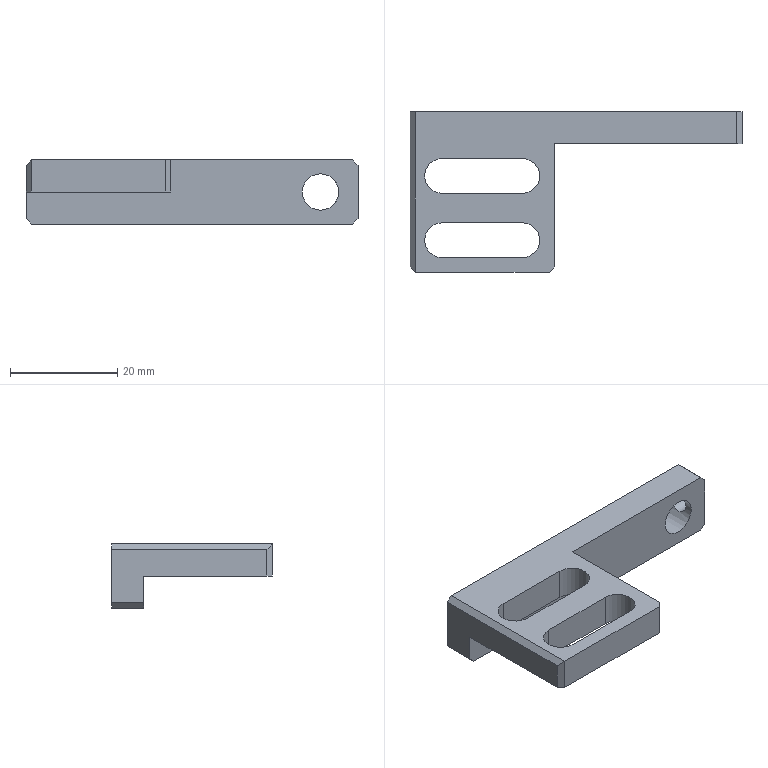Part | NX | 1 solid | 25 faces | box 62 x 30 x 12 mm | volume 6504 mm3 | plane 19 | cylinder 6 | commonest cylinder face diameters 6.5 x4 3.3 x1 6.8 x1
STEP:
#1=CARTESIAN_POINT('',(24.,9.,-2.6));
#2=VERTEX_POINT('',#1);
#3=CARTESIAN_POINT('',(24.,9.,-6.));
#4=DIRECTION('',(0.,1.,0.));
#5=DIRECTION('',(0.,0.,1.));
#6=AXIS2_PLACEMENT_3D('',#3,#4,#5);
#7=CIRCLE('',#6,3.4);
#8=EDGE_CURVE('',#2,#2,#7,.F.);
#9=ORIENTED_EDGE('',*,*,#8,.F.);
#10=EDGE_LOOP('',(#9));
#11=FACE_BOUND('',#10,.T.);
#12=CARTESIAN_POINT('',(31.,9.,-11.));
#13=VERTEX_POINT('',#12);
#14=CARTESIAN_POINT('',(31.,9.,-1.));
#15=VERTEX_POINT('',#14);
#16=CARTESIAN_POINT('',(31.,9.,0.));
#17=DIRECTION('',(0.,0.,-1.));
#18=VECTOR('',#17,1000.);
#19=LINE('',#16,#18);
#20=EDGE_CURVE('',#13,#15,#19,.F.);
#21=ORIENTED_EDGE('',*,*,#20,.T.);
#22=CARTESIAN_POINT('',(30.,9.,0.));
#23=VERTEX_POINT('',#22);
#24=CARTESIAN_POINT('',(30.,9.,0.));
#25=DIRECTION('',(-0.7071,0.,0.7071));
#26=VECTOR('',#25,1000.);
#27=LINE('',#24,#26);
#28=EDGE_CURVE('',#15,#23,#27,.T.);
#29=ORIENTED_EDGE('',*,*,#28,.T.);
#30=CARTESIAN_POINT('',(-4.,9.,0.));
#31=VERTEX_POINT('',#30);
#32=CARTESIAN_POINT('',(-31.,9.,0.));
#33=DIRECTION('',(1.,0.,0.));
#34=VECTOR('',#33,1000.);
#35=LINE('',#32,#34);
#36=EDGE_CURVE('',#31,#23,#35,.T.);
#37=ORIENTED_EDGE('',*,*,#36,.F.);
#38=CARTESIAN_POINT('',(-4.,9.,-6.));
#39=VERTEX_POINT('',#38);
#40=CARTESIAN_POINT('',(-4.,9.,-6.));
#41=DIRECTION('',(0.,0.,1.));
#42=VECTOR('',#41,1000.);
#43=LINE('',#40,#42);
#44=EDGE_CURVE('',#31,#39,#43,.F.);
#45=ORIENTED_EDGE('',*,*,#44,.T.);
#46=CARTESIAN_POINT('',(-31.,9.,-6.));
#47=VERTEX_POINT('',#46);
#48=CARTESIAN_POINT('',(-31.,9.,-6.));
#49=DIRECTION('',(1.,0.,0.));
#50=VECTOR('',#49,1000.);
#51=LINE('',#48,#50);
#52=EDGE_CURVE('',#39,#47,#51,.F.);
#53=ORIENTED_EDGE('',*,*,#52,.T.);
#54=CARTESIAN_POINT('',(-31.,9.,-11.));
#55=VERTEX_POINT('',#54);
#56=CARTESIAN_POINT('',(-31.,9.,0.));
#57=DIRECTION('',(0.,0.,-1.));
#58=VECTOR('',#57,1000.);
#59=LINE('',#56,#58);
#60=EDGE_CURVE('',#47,#55,#59,.T.);
#61=ORIENTED_EDGE('',*,*,#60,.T.);
#62=CARTESIAN_POINT('',(-30.,9.,-12.));
#63=VERTEX_POINT('',#62);
#64=CARTESIAN_POINT('',(-31.,9.,-11.));
#65=DIRECTION('',(-0.7071,0.,0.7071));
#66=VECTOR('',#65,1000.);
#67=LINE('',#64,#66);
#68=EDGE_CURVE('',#55,#63,#67,.F.);
#69=ORIENTED_EDGE('',*,*,#68,.T.);
#70=CARTESIAN_POINT('',(30.,9.,-12.));
#71=VERTEX_POINT('',#70);
#72=CARTESIAN_POINT('',(-4.,9.,-12.));
#73=DIRECTION('',(1.,0.,0.));
#74=VECTOR('',#73,1000.);
#75=LINE('',#72,#74);
#76=EDGE_CURVE('',#63,#71,#75,.T.);
#77=ORIENTED_EDGE('',*,*,#76,.T.);
#78=CARTESIAN_POINT('',(31.,9.,-11.));
#79=DIRECTION('',(-0.7071,0.,-0.7071));
#80=VECTOR('',#79,1000.);
#81=LINE('',#78,#80);
#82=EDGE_CURVE('',#71,#13,#81,.F.);
#83=ORIENTED_EDGE('',*,*,#82,.T.);
#84=EDGE_LOOP('',(#21,#29,#37,#45,#53,#61,#69,#77,#83));
#85=FACE_BOUND('',#84,.T.);
#86=CARTESIAN_POINT('',(-4.,9.,0.));
#87=DIRECTION('',(0.,1.,0.));
#88=DIRECTION('',(0.,0.,1.));
#89=AXIS2_PLACEMENT_3D('',#86,#87,#88);
#90=PLANE('',#89);
#91=ADVANCED_FACE('',(#11,#85),#90,.F.);
#92=CARTESIAN_POINT('',(31.,13.65,-6.));
#93=VERTEX_POINT('',#92);
#94=CARTESIAN_POINT('',(31.,12.,-6.));
#95=DIRECTION('',(1.,0.,0.));
#96=DIRECTION('',(0.,1.,0.));
#97=AXIS2_PLACEMENT_3D('',#94,#95,#96);
#98=CIRCLE('',#97,1.65);
#99=EDGE_CURVE('',#93,#93,#98,.T.);
#100=ORIENTED_EDGE('',*,*,#99,.F.);
#101=EDGE_LOOP('',(#100));
#102=FACE_BOUND('',#101,.T.);
#103=CARTESIAN_POINT('',(31.,15.,-11.));
#104=VERTEX_POINT('',#103);
#105=CARTESIAN_POINT('',(31.,15.,-1.));
#106=VERTEX_POINT('',#105);
#107=CARTESIAN_POINT('',(31.,15.,0.));
#108=DIRECTION('',(0.,0.,-1.));
#109=VECTOR('',#108,1000.);
#110=LINE('',#107,#109);
#111=EDGE_CURVE('',#104,#106,#110,.F.);
#112=ORIENTED_EDGE('',*,*,#111,.T.);
#113=CARTESIAN_POINT('',(31.,9.,-1.));
#114=DIRECTION('',(0.,-1.,0.));
#115=VECTOR('',#114,1000.);
#116=LINE('',#113,#115);
#117=EDGE_CURVE('',#106,#15,#116,.T.);
#118=ORIENTED_EDGE('',*,*,#117,.T.);
#119=ORIENTED_EDGE('',*,*,#20,.F.);
#120=CARTESIAN_POINT('',(31.,13.65,-11.));
#121=DIRECTION('',(0.,1.,0.));
#122=VECTOR('',#121,1000.);
#123=LINE('',#120,#122);
#124=EDGE_CURVE('',#13,#104,#123,.T.);
#125=ORIENTED_EDGE('',*,*,#124,.T.);
#126=EDGE_LOOP('',(#112,#118,#119,#125));
#127=FACE_BOUND('',#126,.T.);
#128=CARTESIAN_POINT('',(31.,13.65,0.));
#129=DIRECTION('',(-1.,0.,0.));
#130=DIRECTION('',(0.,0.,1.));
#131=AXIS2_PLACEMENT_3D('',#128,#129,#130);
#132=PLANE('',#131);
#133=ADVANCED_FACE('',(#102,#127),#132,.F.);
#134=CARTESIAN_POINT('',(24.,15.,-9.4));
#135=VERTEX_POINT('',#134);
#136=CARTESIAN_POINT('',(24.,15.,-6.));
#137=DIRECTION('',(0.,-1.,0.));
#138=DIRECTION('',(0.,0.,-1.));
#139=AXIS2_PLACEMENT_3D('',#136,#137,#138);
#140=CIRCLE('',#139,3.4);
#141=EDGE_CURVE('',#135,#135,#140,.F.);
#142=ORIENTED_EDGE('',*,*,#141,.F.);
#143=EDGE_LOOP('',(#142));
#144=FACE_BOUND('',#143,.T.);
#145=CARTESIAN_POINT('',(30.,15.,0.));
#146=VERTEX_POINT('',#145);
#147=CARTESIAN_POINT('',(-30.,15.,0.));
#148=VERTEX_POINT('',#147);
#149=CARTESIAN_POINT('',(31.,15.,0.));
#150=DIRECTION('',(-1.,0.,0.));
#151=VECTOR('',#150,1000.);
#152=LINE('',#149,#151);
#153=EDGE_CURVE('',#146,#148,#152,.T.);
#154=ORIENTED_EDGE('',*,*,#153,.F.);
#155=CARTESIAN_POINT('',(30.,15.,0.));
#156=DIRECTION('',(0.7071,0.,-0.7071));
#157=VECTOR('',#156,1000.);
#158=LINE('',#155,#157);
#159=EDGE_CURVE('',#146,#106,#158,.T.);
#160=ORIENTED_EDGE('',*,*,#159,.T.);
#161=ORIENTED_EDGE('',*,*,#111,.F.);
#162=CARTESIAN_POINT('',(30.,15.,-12.));
#163=VERTEX_POINT('',#162);
#164=CARTESIAN_POINT('',(31.,15.,-11.));
#165=DIRECTION('',(0.7071,0.,0.7071));
#166=VECTOR('',#165,1000.);
#167=LINE('',#164,#166);
#168=EDGE_CURVE('',#104,#163,#167,.F.);
#169=ORIENTED_EDGE('',*,*,#168,.T.);
#170=CARTESIAN_POINT('',(-30.,15.,-12.));
#171=VERTEX_POINT('',#170);
#172=CARTESIAN_POINT('',(31.,15.,-12.));
#173=DIRECTION('',(-1.,0.,0.));
#174=VECTOR('',#173,1000.);
#175=LINE('',#172,#174);
#176=EDGE_CURVE('',#163,#171,#175,.T.);
#177=ORIENTED_EDGE('',*,*,#176,.T.);
#178=CARTESIAN_POINT('',(-31.,15.,-11.));
#179=VERTEX_POINT('',#178);
#180=CARTESIAN_POINT('',(-31.,15.,-11.));
#181=DIRECTION('',(0.7071,0.,-0.7071));
#182=VECTOR('',#181,1000.);
#183=LINE('',#180,#182);
#184=EDGE_CURVE('',#171,#179,#183,.F.);
#185=ORIENTED_EDGE('',*,*,#184,.T.);
#186=CARTESIAN_POINT('',(-31.,15.,-1.));
#187=VERTEX_POINT('',#186);
#188=CARTESIAN_POINT('',(-31.,15.,0.));
#189=DIRECTION('',(0.,0.,-1.));
#190=VECTOR('',#189,1000.);
#191=LINE('',#188,#190);
#192=EDGE_CURVE('',#179,#187,#191,.F.);
#193=ORIENTED_EDGE('',*,*,#192,.T.);
#194=CARTESIAN_POINT('',(-30.,15.,0.));
#195=DIRECTION('',(0.7071,0.,0.7071));
#196=VECTOR('',#195,1000.);
#197=LINE('',#194,#196);
#198=EDGE_CURVE('',#187,#148,#197,.T.);
#199=ORIENTED_EDGE('',*,*,#198,.T.);
#200=EDGE_LOOP('',(#154,#160,#161,#169,#177,#185,#193,#199));
#201=FACE_BOUND('',#200,.T.);
#202=CARTESIAN_POINT('',(31.,15.,0.));
#203=DIRECTION('',(0.,-1.,0.));
#204=DIRECTION('',(0.,0.,-1.));
#205=AXIS2_PLACEMENT_3D('',#202,#203,#204);
#206=PLANE('',#205);
#207=ADVANCED_FACE('',(#144,#201),#206,.F.);
#208=CARTESIAN_POINT('',(-31.,-14.,-1.));
#209=VERTEX_POINT('',#208);
#210=CARTESIAN_POINT('',(-31.,-14.,-6.));
#211=VERTEX_POINT('',#210);
#212=CARTESIAN_POINT('',(-31.,-14.,-6.));
#213=DIRECTION('',(0.,0.,1.));
#214=VECTOR('',#213,1000.);
#215=LINE('',#212,#214);
#216=EDGE_CURVE('',#209,#211,#215,.F.);
#217=ORIENTED_EDGE('',*,*,#216,.F.);
#218=CARTESIAN_POINT('',(-31.,15.,-1.));
#219=DIRECTION('',(0.,1.,0.));
#220=VECTOR('',#219,1000.);
#221=LINE('',#218,#220);
#222=EDGE_CURVE('',#209,#187,#221,.T.);
#223=ORIENTED_EDGE('',*,*,#222,.T.);
#224=ORIENTED_EDGE('',*,*,#192,.F.);
#225=CARTESIAN_POINT('',(-31.,15.,-11.));
#226=DIRECTION('',(0.,-1.,0.));
#227=VECTOR('',#226,1000.);
#228=LINE('',#225,#227);
#229=EDGE_CURVE('',#179,#55,#228,.T.);
#230=ORIENTED_EDGE('',*,*,#229,.T.);
#231=ORIENTED_EDGE('',*,*,#60,.F.);
#232=CARTESIAN_POINT('',(-31.,-14.,-6.));
#233=DIRECTION('',(0.,1.,0.));
#234=VECTOR('',#233,1000.);
#235=LINE('',#232,#234);
#236=EDGE_CURVE('',#47,#211,#235,.F.);
#237=ORIENTED_EDGE('',*,*,#236,.T.);
#238=EDGE_LOOP('',(#217,#223,#224,#230,#231,#237));
#239=FACE_BOUND('',#238,.T.);
#240=CARTESIAN_POINT('',(-31.,15.,0.));
#241=DIRECTION('',(1.,0.,0.));
#242=DIRECTION('',(0.,0.,-1.));
#243=AXIS2_PLACEMENT_3D('',#240,#241,#242);
#244=PLANE('',#243);
#245=ADVANCED_FACE('',(#239),#244,.F.);
#246=ORIENTED_EDGE('',*,*,#36,.T.);
#247=CARTESIAN_POINT('',(30.,15.,0.));
#248=DIRECTION('',(0.,1.,0.));
#249=VECTOR('',#248,1000.);
#250=LINE('',#247,#249);
#251=EDGE_CURVE('',#23,#146,#250,.T.);
#252=ORIENTED_EDGE('',*,*,#251,.T.);
#253=ORIENTED_EDGE('',*,*,#153,.T.);
#254=CARTESIAN_POINT('',(-30.,-15.,0.));
#255=VERTEX_POINT('',#254);
#256=CARTESIAN_POINT('',(-30.,-14.,0.));
#257=DIRECTION('',(0.,-1.,0.));
#258=VECTOR('',#257,1000.);
#259=LINE('',#256,#258);
#260=EDGE_CURVE('',#148,#255,#259,.T.);
#261=ORIENTED_EDGE('',*,*,#260,.T.);
#262=CARTESIAN_POINT('',(-5.,-15.,0.));
#263=VERTEX_POINT('',#262);
#264=CARTESIAN_POINT('',(-5.,-15.,0.));
#265=DIRECTION('',(-1.,0.,0.));
#266=VECTOR('',#265,1000.);
#267=LINE('',#264,#266);
#268=EDGE_CURVE('',#255,#263,#267,.F.);
#269=ORIENTED_EDGE('',*,*,#268,.T.);
#270=CARTESIAN_POINT('',(-4.,-14.,0.));
#271=VERTEX_POINT('',#270);
#272=CARTESIAN_POINT('',(-4.,-14.,0.));
#273=DIRECTION('',(-0.7071,-0.7071,0.));
#274=VECTOR('',#273,1000.);
#275=LINE('',#272,#274);
#276=EDGE_CURVE('',#263,#271,#275,.F.);
#277=ORIENTED_EDGE('',*,*,#276,.T.);
#278=CARTESIAN_POINT('',(-4.,9.,0.));
#279=DIRECTION('',(0.,-1.,0.));
#280=VECTOR('',#279,1000.);
#281=LINE('',#278,#280);
#282=EDGE_CURVE('',#271,#31,#281,.F.);
#283=ORIENTED_EDGE('',*,*,#282,.T.);
#284=EDGE_LOOP('',(#246,#252,#253,#261,#269,#277,#283));
#285=FACE_BOUND('',#284,.T.);
#286=CARTESIAN_POINT('',(-25.,-0.25,0.));
#287=VERTEX_POINT('',#286);
#288=CARTESIAN_POINT('',(-10.,-0.25,0.));
#289=VERTEX_POINT('',#288);
#290=CARTESIAN_POINT('',(-10.,-0.25,0.));
#291=DIRECTION('',(-1.,0.,0.));
#292=VECTOR('',#291,1000.);
#293=LINE('',#290,#292);
#294=EDGE_CURVE('',#287,#289,#293,.F.);
#295=ORIENTED_EDGE('',*,*,#294,.F.);
#296=CARTESIAN_POINT('',(-25.,6.25,0.));
#297=VERTEX_POINT('',#296);
#298=CARTESIAN_POINT('',(-25.,3.,0.));
#299=DIRECTION('',(0.,0.,-1.));
#300=DIRECTION('',(0.,1.,0.));
#301=AXIS2_PLACEMENT_3D('',#298,#299,#300);
#302=CIRCLE('',#301,3.25);
#303=EDGE_CURVE('',#297,#287,#302,.F.);
#304=ORIENTED_EDGE('',*,*,#303,.F.);
#305=CARTESIAN_POINT('',(-10.,6.25,0.));
#306=VERTEX_POINT('',#305);
#307=CARTESIAN_POINT('',(-25.,6.25,0.));
#308=DIRECTION('',(1.,0.,0.));
#309=VECTOR('',#308,1000.);
#310=LINE('',#307,#309);
#311=EDGE_CURVE('',#306,#297,#310,.F.);
#312=ORIENTED_EDGE('',*,*,#311,.F.);
#313=CARTESIAN_POINT('',(-10.,3.,0.));
#314=DIRECTION('',(0.,0.,-1.));
#315=DIRECTION('',(0.,1.,0.));
#316=AXIS2_PLACEMENT_3D('',#313,#314,#315);
#317=CIRCLE('',#316,3.25);
#318=EDGE_CURVE('',#289,#306,#317,.F.);
#319=ORIENTED_EDGE('',*,*,#318,.F.);
#320=EDGE_LOOP('',(#295,#304,#312,#319));
#321=FACE_BOUND('',#320,.T.);
#322=CARTESIAN_POINT('',(-25.,-12.25,0.));
#323=VERTEX_POINT('',#322);
#324=CARTESIAN_POINT('',(-10.,-12.25,0.));
#325=VERTEX_POINT('',#324);
#326=CARTESIAN_POINT('',(-10.,-12.25,0.));
#327=DIRECTION('',(-1.,0.,0.));
#328=VECTOR('',#327,1000.);
#329=LINE('',#326,#328);
#330=EDGE_CURVE('',#323,#325,#329,.F.);
#331=ORIENTED_EDGE('',*,*,#330,.F.);
#332=CARTESIAN_POINT('',(-25.,-5.75,0.));
#333=VERTEX_POINT('',#332);
#334=CARTESIAN_POINT('',(-25.,-9.,0.));
#335=DIRECTION('',(0.,0.,-1.));
#336=DIRECTION('',(0.,1.,0.));
#337=AXIS2_PLACEMENT_3D('',#334,#335,#336);
#338=CIRCLE('',#337,3.25);
#339=EDGE_CURVE('',#333,#323,#338,.F.);
#340=ORIENTED_EDGE('',*,*,#339,.F.);
#341=CARTESIAN_POINT('',(-10.,-5.75,0.));
#342=VERTEX_POINT('',#341);
#343=CARTESIAN_POINT('',(-25.,-5.75,0.));
#344=DIRECTION('',(1.,0.,0.));
#345=VECTOR('',#344,1000.);
#346=LINE('',#343,#345);
#347=EDGE_CURVE('',#342,#333,#346,.F.);
#348=ORIENTED_EDGE('',*,*,#347,.F.);
#349=CARTESIAN_POINT('',(-10.,-9.,0.));
#350=DIRECTION('',(0.,0.,-1.));
#351=DIRECTION('',(0.,1.,0.));
#352=AXIS2_PLACEMENT_3D('',#349,#350,#351);
#353=CIRCLE('',#352,3.25);
#354=EDGE_CURVE('',#325,#342,#353,.F.);
#355=ORIENTED_EDGE('',*,*,#354,.F.);
#356=EDGE_LOOP('',(#331,#340,#348,#355));
#357=FACE_BOUND('',#356,.T.);
#358=CARTESIAN_POINT('',(-115.031,-113.478,0.));
#359=DIRECTION('',(0.,0.,1.));
#360=DIRECTION('',(0.,-1.,0.));
#361=AXIS2_PLACEMENT_3D('',#358,#359,#360);
#362=PLANE('',#361);
#363=ADVANCED_FACE('',(#285,#321,#357),#362,.T.);
#364=ORIENTED_EDGE('',*,*,#176,.F.);
#365=CARTESIAN_POINT('',(30.,-113.478,-12.));
#366=DIRECTION('',(0.,-1.,0.));
#367=VECTOR('',#366,1000.);
#368=LINE('',#365,#367);
#369=EDGE_CURVE('',#163,#71,#368,.T.);
#370=ORIENTED_EDGE('',*,*,#369,.T.);
#371=ORIENTED_EDGE('',*,*,#76,.F.);
#372=CARTESIAN_POINT('',(-30.,-113.478,-12.));
#373=DIRECTION('',(0.,1.,0.));
#374=VECTOR('',#373,1000.);
#375=LINE('',#372,#374);
#376=EDGE_CURVE('',#63,#171,#375,.T.);
#377=ORIENTED_EDGE('',*,*,#376,.T.);
#378=EDGE_LOOP('',(#364,#370,#371,#377));
#379=FACE_BOUND('',#378,.T.);
#380=CARTESIAN_POINT('',(-115.031,-113.478,-12.));
#381=DIRECTION('',(0.,0.,1.));
#382=DIRECTION('',(0.,-1.,0.));
#383=AXIS2_PLACEMENT_3D('',#380,#381,#382);
#384=PLANE('',#383);
#385=ADVANCED_FACE('',(#379),#384,.F.);
#386=ORIENTED_EDGE('',*,*,#330,.T.);
#387=CARTESIAN_POINT('',(-10.,-12.25,-6.));
#388=VERTEX_POINT('',#387);
#389=CARTESIAN_POINT('',(-10.,-12.25,-6.));
#390=DIRECTION('',(0.,0.,1.));
#391=VECTOR('',#390,1000.);
#392=LINE('',#389,#391);
#393=EDGE_CURVE('',#325,#388,#392,.F.);
#394=ORIENTED_EDGE('',*,*,#393,.T.);
#395=CARTESIAN_POINT('',(-25.,-12.25,-6.));
#396=VERTEX_POINT('',#395);
#397=CARTESIAN_POINT('',(-10.,-12.25,-6.));
#398=DIRECTION('',(-1.,0.,0.));
#399=VECTOR('',#398,1000.);
#400=LINE('',#397,#399);
#401=EDGE_CURVE('',#396,#388,#400,.F.);
#402=ORIENTED_EDGE('',*,*,#401,.F.);
#403=CARTESIAN_POINT('',(-25.,-12.25,-6.));
#404=DIRECTION('',(0.,0.,1.));
#405=VECTOR('',#404,1000.);
#406=LINE('',#403,#405);
#407=EDGE_CURVE('',#323,#396,#406,.F.);
#408=ORIENTED_EDGE('',*,*,#407,.F.);
#409=EDGE_LOOP('',(#386,#394,#402,#408));
#410=FACE_BOUND('',#409,.T.);
#411=CARTESIAN_POINT('',(-10.,-12.25,-6.));
#412=DIRECTION('',(0.,1.,0.));
#413=DIRECTION('',(0.,0.,1.));
#414=AXIS2_PLACEMENT_3D('',#411,#412,#413);
#415=PLANE('',#414);
#416=ADVANCED_FACE('',(#410),#415,.T.);
#417=ORIENTED_EDGE('',*,*,#354,.T.);
#418=CARTESIAN_POINT('',(-10.,-5.75,-6.));
#419=VERTEX_POINT('',#418);
#420=CARTESIAN_POINT('',(-10.,-5.75,-6.));
#421=DIRECTION('',(0.,0.,1.));
#422=VECTOR('',#421,1000.);
#423=LINE('',#420,#422);
#424=EDGE_CURVE('',#342,#419,#423,.F.);
#425=ORIENTED_EDGE('',*,*,#424,.T.);
#426=CARTESIAN_POINT('',(-10.,-9.,-6.));
#427=DIRECTION('',(0.,0.,-1.));
#428=DIRECTION('',(0.,1.,0.));
#429=AXIS2_PLACEMENT_3D('',#426,#427,#428);
#430=CIRCLE('',#429,3.25);
#431=EDGE_CURVE('',#388,#419,#430,.F.);
#432=ORIENTED_EDGE('',*,*,#431,.F.);
#433=ORIENTED_EDGE('',*,*,#393,.F.);
#434=EDGE_LOOP('',(#417,#425,#432,#433));
#435=FACE_BOUND('',#434,.T.);
#436=CARTESIAN_POINT('',(-10.,-9.,-6.));
#437=DIRECTION('',(0.,0.,1.));
#438=DIRECTION('',(0.,-1.,0.));
#439=AXIS2_PLACEMENT_3D('',#436,#437,#438);
#440=CYLINDRICAL_SURFACE('',#439,3.25);
#441=ADVANCED_FACE('',(#435),#440,.F.);
#442=ORIENTED_EDGE('',*,*,#347,.T.);
#443=CARTESIAN_POINT('',(-25.,-5.75,-6.));
#444=VERTEX_POINT('',#443);
#445=CARTESIAN_POINT('',(-25.,-5.75,-6.));
#446=DIRECTION('',(0.,0.,1.));
#447=VECTOR('',#446,1000.);
#448=LINE('',#445,#447);
#449=EDGE_CURVE('',#333,#444,#448,.F.);
#450=ORIENTED_EDGE('',*,*,#449,.T.);
#451=CARTESIAN_POINT('',(-25.,-5.75,-6.));
#452=DIRECTION('',(1.,0.,0.));
#453=VECTOR('',#452,1000.);
#454=LINE('',#451,#453);
#455=EDGE_CURVE('',#419,#444,#454,.F.);
#456=ORIENTED_EDGE('',*,*,#455,.F.);
#457=ORIENTED_EDGE('',*,*,#424,.F.);
#458=EDGE_LOOP('',(#442,#450,#456,#457));
#459=FACE_BOUND('',#458,.T.);
#460=CARTESIAN_POINT('',(-25.,-5.75,-6.));
#461=DIRECTION('',(0.,-1.,0.));
#462=DIRECTION('',(0.,0.,-1.));
#463=AXIS2_PLACEMENT_3D('',#460,#461,#462);
#464=PLANE('',#463);
#465=ADVANCED_FACE('',(#459),#464,.T.);
#466=ORIENTED_EDGE('',*,*,#294,.T.);
#467=CARTESIAN_POINT('',(-10.,-0.25,-6.));
#468=VERTEX_POINT('',#467);
#469=CARTESIAN_POINT('',(-10.,-0.25,-6.));
#470=DIRECTION('',(0.,0.,1.));
#471=VECTOR('',#470,1000.);
#472=LINE('',#469,#471);
#473=EDGE_CURVE('',#289,#468,#472,.F.);
#474=ORIENTED_EDGE('',*,*,#473,.T.);
#475=CARTESIAN_POINT('',(-25.,-0.25,-6.));
#476=VERTEX_POINT('',#475);
#477=CARTESIAN_POINT('',(-10.,-0.25,-6.));
#478=DIRECTION('',(-1.,0.,0.));
#479=VECTOR('',#478,1000.);
#480=LINE('',#477,#479);
#481=EDGE_CURVE('',#476,#468,#480,.F.);
#482=ORIENTED_EDGE('',*,*,#481,.F.);
#483=CARTESIAN_POINT('',(-25.,-0.25,-6.));
#484=DIRECTION('',(0.,0.,1.));
#485=VECTOR('',#484,1000.);
#486=LINE('',#483,#485);
#487=EDGE_CURVE('',#287,#476,#486,.F.);
#488=ORIENTED_EDGE('',*,*,#487,.F.);
#489=EDGE_LOOP('',(#466,#474,#482,#488));
#490=FACE_BOUND('',#489,.T.);
#491=CARTESIAN_POINT('',(-10.,-0.25,-6.));
#492=DIRECTION('',(0.,1.,0.));
#493=DIRECTION('',(0.,0.,1.));
#494=AXIS2_PLACEMENT_3D('',#491,#492,#493);
#495=PLANE('',#494);
#496=ADVANCED_FACE('',(#490),#495,.T.);
#497=ORIENTED_EDGE('',*,*,#318,.T.);
#498=CARTESIAN_POINT('',(-10.,6.25,-6.));
#499=VERTEX_POINT('',#498);
#500=CARTESIAN_POINT('',(-10.,6.25,-6.));
#501=DIRECTION('',(0.,0.,1.));
#502=VECTOR('',#501,1000.);
#503=LINE('',#500,#502);
#504=EDGE_CURVE('',#306,#499,#503,.F.);
#505=ORIENTED_EDGE('',*,*,#504,.T.);
#506=CARTESIAN_POINT('',(-10.,3.,-6.));
#507=DIRECTION('',(0.,0.,-1.));
#508=DIRECTION('',(0.,1.,0.));
#509=AXIS2_PLACEMENT_3D('',#506,#507,#508);
#510=CIRCLE('',#509,3.25);
#511=EDGE_CURVE('',#468,#499,#510,.F.);
#512=ORIENTED_EDGE('',*,*,#511,.F.);
#513=ORIENTED_EDGE('',*,*,#473,.F.);
#514=EDGE_LOOP('',(#497,#505,#512,#513));
#515=FACE_BOUND('',#514,.T.);
#516=CARTESIAN_POINT('',(-10.,3.,-6.));
#517=DIRECTION('',(0.,0.,1.));
#518=DIRECTION('',(0.,-1.,0.));
#519=AXIS2_PLACEMENT_3D('',#516,#517,#518);
#520=CYLINDRICAL_SURFACE('',#519,3.25);
#521=ADVANCED_FACE('',(#515),#520,.F.);
#522=ORIENTED_EDGE('',*,*,#311,.T.);
#523=CARTESIAN_POINT('',(-25.,6.25,-6.));
#524=VERTEX_POINT('',#523);
#525=CARTESIAN_POINT('',(-25.,6.25,-6.));
#526=DIRECTION('',(0.,0.,1.));
#527=VECTOR('',#526,1000.);
#528=LINE('',#525,#527);
#529=EDGE_CURVE('',#297,#524,#528,.F.);
#530=ORIENTED_EDGE('',*,*,#529,.T.);
#531=CARTESIAN_POINT('',(-25.,6.25,-6.));
#532=DIRECTION('',(1.,0.,0.));
#533=VECTOR('',#532,1000.);
#534=LINE('',#531,#533);
#535=EDGE_CURVE('',#499,#524,#534,.F.);
#536=ORIENTED_EDGE('',*,*,#535,.F.);
#537=ORIENTED_EDGE('',*,*,#504,.F.);
#538=EDGE_LOOP('',(#522,#530,#536,#537));
#539=FACE_BOUND('',#538,.T.);
#540=CARTESIAN_POINT('',(-25.,6.25,-6.));
#541=DIRECTION('',(0.,-1.,0.));
#542=DIRECTION('',(0.,0.,-1.));
#543=AXIS2_PLACEMENT_3D('',#540,#541,#542);
#544=PLANE('',#543);
#545=ADVANCED_FACE('',(#539),#544,.T.);
#546=ORIENTED_EDGE('',*,*,#282,.F.);
#547=CARTESIAN_POINT('',(-4.,-14.,-6.));
#548=VERTEX_POINT('',#547);
#549=CARTESIAN_POINT('',(-4.,-14.,-6.));
#550=DIRECTION('',(0.,0.,1.));
#551=VECTOR('',#550,1000.);
#552=LINE('',#549,#551);
#553=EDGE_CURVE('',#271,#548,#552,.F.);
#554=ORIENTED_EDGE('',*,*,#553,.T.);
#555=CARTESIAN_POINT('',(-4.,9.,-6.));
#556=DIRECTION('',(0.,-1.,0.));
#557=VECTOR('',#556,1000.);
#558=LINE('',#555,#557);
#559=EDGE_CURVE('',#548,#39,#558,.F.);
#560=ORIENTED_EDGE('',*,*,#559,.T.);
#561=ORIENTED_EDGE('',*,*,#44,.F.);
#562=EDGE_LOOP('',(#546,#554,#560,#561));
#563=FACE_BOUND('',#562,.T.);
#564=CARTESIAN_POINT('',(-4.,9.,-6.));
#565=DIRECTION('',(-1.,0.,0.));
#566=DIRECTION('',(0.,0.,1.));
#567=AXIS2_PLACEMENT_3D('',#564,#565,#566);
#568=PLANE('',#567);
#569=ADVANCED_FACE('',(#563),#568,.F.);
#570=ORIENTED_EDGE('',*,*,#276,.F.);
#571=CARTESIAN_POINT('',(-5.,-15.,-6.));
#572=VERTEX_POINT('',#571);
#573=CARTESIAN_POINT('',(-5.,-15.,-6.));
#574=DIRECTION('',(0.,0.,1.));
#575=VECTOR('',#574,1000.);
#576=LINE('',#573,#575);
#577=EDGE_CURVE('',#263,#572,#576,.F.);
#578=ORIENTED_EDGE('',*,*,#577,.T.);
#579=CARTESIAN_POINT('',(-4.,-14.,-6.));
#580=DIRECTION('',(-0.7071,-0.7071,0.));
#581=VECTOR('',#580,1000.);
#582=LINE('',#579,#581);
#583=EDGE_CURVE('',#572,#548,#582,.F.);
#584=ORIENTED_EDGE('',*,*,#583,.T.);
#585=ORIENTED_EDGE('',*,*,#553,.F.);
#586=EDGE_LOOP('',(#570,#578,#584,#585));
#587=FACE_BOUND('',#586,.T.);
#588=CARTESIAN_POINT('',(-4.,-14.,-6.));
#589=DIRECTION('',(-0.7071,0.7071,0.));
#590=DIRECTION('',(0.7071,0.7071,0.));
#591=AXIS2_PLACEMENT_3D('',#588,#589,#590);
#592=PLANE('',#591);
#593=ADVANCED_FACE('',(#587),#592,.F.);
#594=ORIENTED_EDGE('',*,*,#268,.F.);
#595=CARTESIAN_POINT('',(-30.,-15.,-6.));
#596=VERTEX_POINT('',#595);
#597=CARTESIAN_POINT('',(-30.,-15.,-6.));
#598=DIRECTION('',(0.,0.,1.));
#599=VECTOR('',#598,1000.);
#600=LINE('',#597,#599);
#601=EDGE_CURVE('',#255,#596,#600,.F.);
#602=ORIENTED_EDGE('',*,*,#601,.T.);
#603=CARTESIAN_POINT('',(-5.,-15.,-6.));
#604=DIRECTION('',(-1.,0.,0.));
#605=VECTOR('',#604,1000.);
#606=LINE('',#603,#605);
#607=EDGE_CURVE('',#596,#572,#606,.F.);
#608=ORIENTED_EDGE('',*,*,#607,.T.);
#609=ORIENTED_EDGE('',*,*,#577,.F.);
#610=EDGE_LOOP('',(#594,#602,#608,#609));
#611=FACE_BOUND('',#610,.T.);
#612=CARTESIAN_POINT('',(-5.,-15.,-6.));
#613=DIRECTION('',(0.,1.,0.));
#614=DIRECTION('',(0.,0.,1.));
#615=AXIS2_PLACEMENT_3D('',#612,#613,#614);
#616=PLANE('',#615);
#617=ADVANCED_FACE('',(#611),#616,.F.);
#618=ORIENTED_EDGE('',*,*,#303,.T.);
#619=ORIENTED_EDGE('',*,*,#487,.T.);
#620=CARTESIAN_POINT('',(-25.,3.,-6.));
#621=DIRECTION('',(0.,0.,-1.));
#622=DIRECTION('',(0.,1.,0.));
#623=AXIS2_PLACEMENT_3D('',#620,#621,#622);
#624=CIRCLE('',#623,3.25);
#625=EDGE_CURVE('',#524,#476,#624,.F.);
#626=ORIENTED_EDGE('',*,*,#625,.F.);
#627=ORIENTED_EDGE('',*,*,#529,.F.);
#628=EDGE_LOOP('',(#618,#619,#626,#627));
#629=FACE_BOUND('',#628,.T.);
#630=CARTESIAN_POINT('',(-25.,3.,-6.));
#631=DIRECTION('',(0.,0.,1.));
#632=DIRECTION('',(0.,-1.,0.));
#633=AXIS2_PLACEMENT_3D('',#630,#631,#632);
#634=CYLINDRICAL_SURFACE('',#633,3.25);
#635=ADVANCED_FACE('',(#629),#634,.F.);
#636=ORIENTED_EDGE('',*,*,#601,.F.);
#637=CARTESIAN_POINT('',(2.826,-47.826,32.826));
#638=DIRECTION('',(-0.5774,0.5774,-0.5774));
#639=VECTOR('',#638,1000.);
#640=LINE('',#637,#639);
#641=EDGE_CURVE('',#255,#209,#640,.T.);
#642=ORIENTED_EDGE('',*,*,#641,.T.);
#643=ORIENTED_EDGE('',*,*,#216,.T.);
#644=CARTESIAN_POINT('',(-30.,-15.,-6.));
#645=DIRECTION('',(-0.7071,0.7071,0.));
#646=VECTOR('',#645,1000.);
#647=LINE('',#644,#646);
#648=EDGE_CURVE('',#211,#596,#647,.F.);
#649=ORIENTED_EDGE('',*,*,#648,.T.);
#650=EDGE_LOOP('',(#636,#642,#643,#649));
#651=FACE_BOUND('',#650,.T.);
#652=CARTESIAN_POINT('',(-30.,-15.,-6.));
#653=DIRECTION('',(0.7071,0.7071,0.));
#654=DIRECTION('',(0.7071,-0.7071,0.));
#655=AXIS2_PLACEMENT_3D('',#652,#653,#654);
#656=PLANE('',#655);
#657=ADVANCED_FACE('',(#651),#656,.F.);
#658=ORIENTED_EDGE('',*,*,#339,.T.);
#659=ORIENTED_EDGE('',*,*,#407,.T.);
#660=CARTESIAN_POINT('',(-25.,-9.,-6.));
#661=DIRECTION('',(0.,0.,-1.));
#662=DIRECTION('',(0.,1.,0.));
#663=AXIS2_PLACEMENT_3D('',#660,#661,#662);
#664=CIRCLE('',#663,3.25);
#665=EDGE_CURVE('',#444,#396,#664,.F.);
#666=ORIENTED_EDGE('',*,*,#665,.F.);
#667=ORIENTED_EDGE('',*,*,#449,.F.);
#668=EDGE_LOOP('',(#658,#659,#666,#667));
#669=FACE_BOUND('',#668,.T.);
#670=CARTESIAN_POINT('',(-25.,-9.,-6.));
#671=DIRECTION('',(0.,0.,1.));
#672=DIRECTION('',(0.,-1.,0.));
#673=AXIS2_PLACEMENT_3D('',#670,#671,#672);
#674=CYLINDRICAL_SURFACE('',#673,3.25);
#675=ADVANCED_FACE('',(#669),#674,.F.);
#676=ORIENTED_EDGE('',*,*,#236,.F.);
#677=ORIENTED_EDGE('',*,*,#52,.F.);
#678=ORIENTED_EDGE('',*,*,#559,.F.);
#679=ORIENTED_EDGE('',*,*,#583,.F.);
#680=ORIENTED_EDGE('',*,*,#607,.F.);
#681=ORIENTED_EDGE('',*,*,#648,.F.);
#682=EDGE_LOOP('',(#676,#677,#678,#679,#680,#681));
#683=FACE_BOUND('',#682,.T.);
#684=ORIENTED_EDGE('',*,*,#481,.T.);
#685=ORIENTED_EDGE('',*,*,#511,.T.);
#686=ORIENTED_EDGE('',*,*,#535,.T.);
#687=ORIENTED_EDGE('',*,*,#625,.T.);
#688=EDGE_LOOP('',(#684,#685,#686,#687));
#689=FACE_BOUND('',#688,.T.);
#690=ORIENTED_EDGE('',*,*,#401,.T.);
#691=ORIENTED_EDGE('',*,*,#431,.T.);
#692=ORIENTED_EDGE('',*,*,#455,.T.);
#693=ORIENTED_EDGE('',*,*,#665,.T.);
#694=EDGE_LOOP('',(#690,#691,#692,#693));
#695=FACE_BOUND('',#694,.T.);
#696=CARTESIAN_POINT('',(-10.,3.,-6.));
#697=DIRECTION('',(0.,0.,-1.));
#698=DIRECTION('',(0.,1.,0.));
#699=AXIS2_PLACEMENT_3D('',#696,#697,#698);
#700=PLANE('',#699);
#701=ADVANCED_FACE('',(#683,#689,#695),#700,.T.);
#702=ORIENTED_EDGE('',*,*,#28,.F.);
#703=ORIENTED_EDGE('',*,*,#117,.F.);
#704=ORIENTED_EDGE('',*,*,#159,.F.);
#705=ORIENTED_EDGE('',*,*,#251,.F.);
#706=EDGE_LOOP('',(#702,#703,#704,#705));
#707=FACE_BOUND('',#706,.T.);
#708=CARTESIAN_POINT('',(30.,-113.478,0.));
#709=DIRECTION('',(0.7071,0.,0.7071));
#710=DIRECTION('',(0.,-1.,0.));
#711=AXIS2_PLACEMENT_3D('',#708,#709,#710);
#712=PLANE('',#711);
#713=ADVANCED_FACE('',(#707),#712,.T.);
#714=ORIENTED_EDGE('',*,*,#82,.F.);
#715=ORIENTED_EDGE('',*,*,#369,.F.);
#716=ORIENTED_EDGE('',*,*,#168,.F.);
#717=ORIENTED_EDGE('',*,*,#124,.F.);
#718=EDGE_LOOP('',(#714,#715,#716,#717));
#719=FACE_BOUND('',#718,.T.);
#720=CARTESIAN_POINT('',(31.,13.65,-11.));
#721=DIRECTION('',(-0.7071,0.,0.7071));
#722=DIRECTION('',(0.,1.,0.));
#723=AXIS2_PLACEMENT_3D('',#720,#721,#722);
#724=PLANE('',#723);
#725=ADVANCED_FACE('',(#719),#724,.F.);
#726=ORIENTED_EDGE('',*,*,#198,.F.);
#727=ORIENTED_EDGE('',*,*,#222,.F.);
#728=ORIENTED_EDGE('',*,*,#641,.F.);
#729=ORIENTED_EDGE('',*,*,#260,.F.);
#730=EDGE_LOOP('',(#726,#727,#728,#729));
#731=FACE_BOUND('',#730,.T.);
#732=CARTESIAN_POINT('',(-30.,-113.478,0.));
#733=DIRECTION('',(-0.7071,0.,0.7071));
#734=DIRECTION('',(0.,1.,0.));
#735=AXIS2_PLACEMENT_3D('',#732,#733,#734);
#736=PLANE('',#735);
#737=ADVANCED_FACE('',(#731),#736,.T.);
#738=ORIENTED_EDGE('',*,*,#184,.F.);
#739=ORIENTED_EDGE('',*,*,#376,.F.);
#740=ORIENTED_EDGE('',*,*,#68,.F.);
#741=ORIENTED_EDGE('',*,*,#229,.F.);
#742=EDGE_LOOP('',(#738,#739,#740,#741));
#743=FACE_BOUND('',#742,.T.);
#744=CARTESIAN_POINT('',(-31.,15.,-11.));
#745=DIRECTION('',(0.7071,0.,0.7071));
#746=DIRECTION('',(0.,-1.,0.));
#747=AXIS2_PLACEMENT_3D('',#744,#745,#746);
#748=PLANE('',#747);
#749=ADVANCED_FACE('',(#743),#748,.F.);
#750=CARTESIAN_POINT('',(27.4,13.65,-6.));
#751=VERTEX_POINT('',#750);
#752=CARTESIAN_POINT('',(27.2,13.292,-4.704));
#753=CARTESIAN_POINT('',(27.5,13.829,-6.));
#754=CARTESIAN_POINT('',(27.2,13.291,-7.294));
#755=CARTESIAN_POINT('',(26.859,12.005,-7.828));
#756=CARTESIAN_POINT('',(27.199,10.709,-7.295));
#757=CARTESIAN_POINT('',(27.5,10.171,-6.006));
#758=CARTESIAN_POINT('',(27.201,10.708,-4.706));
#759=CARTESIAN_POINT('',(26.859,11.995,-4.172));
#760=CARTESIAN_POINT('',(27.2,13.292,-4.704));
#761=CARTESIAN_POINT('',(27.5,13.829,-6.));
#762=CARTESIAN_POINT('',(27.2,13.291,-7.294));
#763=B_SPLINE_CURVE_WITH_KNOTS('',3,(#752,#753,#754,#755,#756,#757,#758,#759,#760,#761,#762),.UNSPECIFIED.,.T.,.F.,(1,1,1,1,1,1,1,1,1,1,1,1,1,1,1),(-0.003929,-0.002619,-0.00131,0.,0.00131,0.002619,0.003929,0.005239,0.006548,0.007858,0.009168,0.01048,0.01179,0.0131,0.01441),.UNSPECIFIED.);
#764=EDGE_CURVE('',#751,#751,#763,.T.);
#765=ORIENTED_EDGE('',*,*,#764,.F.);
#766=EDGE_LOOP('',(#765));
#767=FACE_BOUND('',#766,.T.);
#768=ORIENTED_EDGE('',*,*,#141,.T.);
#769=EDGE_LOOP('',(#768));
#770=FACE_BOUND('',#769,.T.);
#771=ORIENTED_EDGE('',*,*,#8,.T.);
#772=EDGE_LOOP('',(#771));
#773=FACE_BOUND('',#772,.T.);
#774=CARTESIAN_POINT('',(24.,-111.715,-6.));
#775=DIRECTION('',(0.,1.,0.));
#776=DIRECTION('',(0.,0.,1.));
#777=AXIS2_PLACEMENT_3D('',#774,#775,#776);
#778=CYLINDRICAL_SURFACE('',#777,3.4);
#779=ADVANCED_FACE('',(#767,#770,#773),#778,.F.);
#780=ORIENTED_EDGE('',*,*,#764,.T.);
#781=EDGE_LOOP('',(#780));
#782=FACE_BOUND('',#781,.T.);
#783=ORIENTED_EDGE('',*,*,#99,.T.);
#784=EDGE_LOOP('',(#783));
#785=FACE_BOUND('',#784,.T.);
#786=CARTESIAN_POINT('',(23.,12.,-6.));
#787=DIRECTION('',(1.,0.,0.));
#788=DIRECTION('',(0.,1.,0.));
#789=AXIS2_PLACEMENT_3D('',#786,#787,#788);
#790=CYLINDRICAL_SURFACE('',#789,1.65);
#791=ADVANCED_FACE('',(#782,#785),#790,.F.);
#792=CLOSED_SHELL('',(#91,#133,#207,#245,#363,#385,#416,#441,#465,#496,#521,#545,#569,#593,#617,#635,#657,#675,#701,#713,#725,#737,#749,#779,#791));
#793=MANIFOLD_SOLID_BREP('',#792);
#794=(LENGTH_UNIT()NAMED_UNIT(*)SI_UNIT(.MILLI.,.METRE.));
#795=UNCERTAINTY_MEASURE_WITH_UNIT(LENGTH_MEASURE(0.0508),#794,'','');
#796=(NAMED_UNIT(*)PLANE_ANGLE_UNIT()SI_UNIT($,.RADIAN.));
#797=(NAMED_UNIT(*)SI_UNIT($,.STERADIAN.)SOLID_ANGLE_UNIT());
#798=(GEOMETRIC_REPRESENTATION_CONTEXT(3)GLOBAL_UNCERTAINTY_ASSIGNED_CONTEXT((#795))GLOBAL_UNIT_ASSIGNED_CONTEXT((#794,#796,#797))REPRESENTATION_CONTEXT('',''));
#799=ADVANCED_BREP_SHAPE_REPRESENTATION('',(#793),#798);